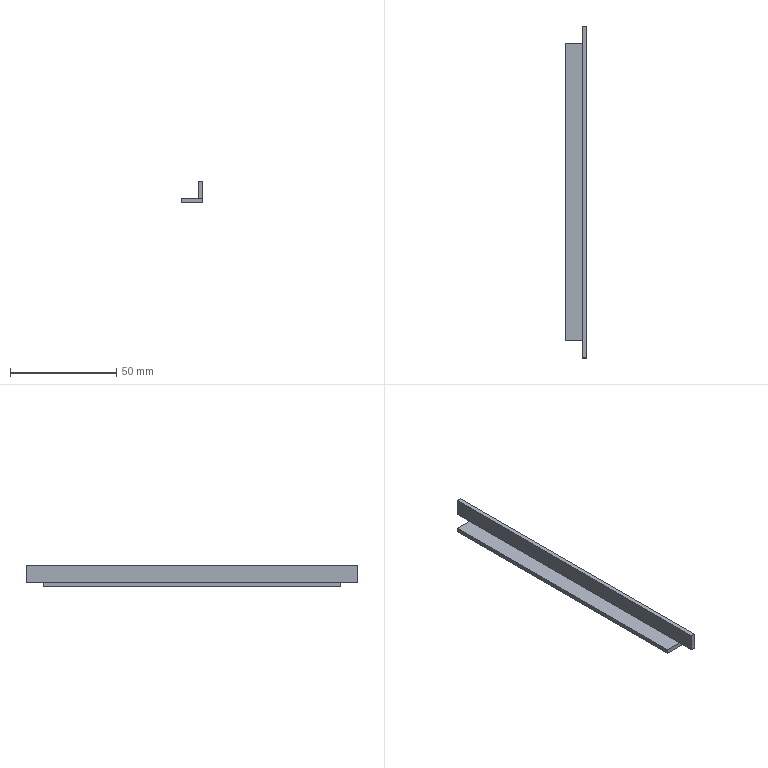Part | STEP file | 1-43.7 | 1 solid | 12 faces | box 10 x 156 x 10 mm | volume 5296 mm3 | plane 12
STEP:
#1=CARTESIAN_POINT('',(0.,0.,0.));
#2=DIRECTION('',(0.,0.,1.));
#3=DIRECTION('',(1.,0.,0.));
#4=AXIS2_PLACEMENT_3D('',#1,#2,#3);
#5=CARTESIAN_POINT('',(3.,-78.,-3.));
#6=VERTEX_POINT('',#5);
#7=CARTESIAN_POINT('',(3.,-78.,5.));
#8=VERTEX_POINT('',#7);
#9=CARTESIAN_POINT('',(3.,-78.,-3.));
#10=DIRECTION('',(0.,0.,1.));
#11=VECTOR('',#10,1.);
#12=LINE('',#9,#11);
#13=CARTESIAN_POINT('',(3.,0.,1.));
#14=DIRECTION('',(-1.,0.,0.));
#15=DIRECTION('',(0.,0.,1.));
#16=AXIS2_PLACEMENT_3D('',#13,#14,#15);
#17=PLANE('',#16);
#18=CARTESIAN_POINT('',(-4.,-78.));
#19=DIRECTION('',(1.,0.));
#20=VECTOR('',#19,1.);
#21=LINE('',#18,#20);
#22=(GEOMETRIC_REPRESENTATION_CONTEXT(2)PARAMETRIC_REPRESENTATION_CONTEXT()REPRESENTATION_CONTEXT('',''));
#23=DEFINITIONAL_REPRESENTATION('',(#21),#22);
#24=PCURVE('',#17,#23);
#25=CARTESIAN_POINT('',(0.,-78.,0.));
#26=DIRECTION('',(0.,1.,0.));
#27=DIRECTION('',(-1.,0.,0.));
#28=AXIS2_PLACEMENT_3D('',#25,#26,#27);
#29=PLANE('',#28);
#30=CARTESIAN_POINT('',(-3.,-3.));
#31=DIRECTION('',(0.,1.));
#32=VECTOR('',#31,1.);
#33=LINE('',#30,#32);
#34=(GEOMETRIC_REPRESENTATION_CONTEXT(2)PARAMETRIC_REPRESENTATION_CONTEXT()REPRESENTATION_CONTEXT('',''));
#35=DEFINITIONAL_REPRESENTATION('',(#33),#34);
#36=PCURVE('',#29,#35);
#37=SURFACE_CURVE('',#12,(#24,#36),.PCURVE_S1.);
#38=EDGE_CURVE('',#6,#8,#37,.T.);
#39=ORIENTED_EDGE('',*,*,#38,.T.);
#40=CARTESIAN_POINT('',(3.,78.,5.));
#41=VERTEX_POINT('',#40);
#42=CARTESIAN_POINT('',(3.,-78.,5.));
#43=DIRECTION('',(0.,1.,0.));
#44=VECTOR('',#43,1.);
#45=LINE('',#42,#44);
#46=CARTESIAN_POINT('',(4.,-78.));
#47=DIRECTION('',(0.,1.));
#48=VECTOR('',#47,1.);
#49=LINE('',#46,#48);
#50=(GEOMETRIC_REPRESENTATION_CONTEXT(2)PARAMETRIC_REPRESENTATION_CONTEXT()REPRESENTATION_CONTEXT('',''));
#51=DEFINITIONAL_REPRESENTATION('',(#49),#50);
#52=PCURVE('',#17,#51);
#53=CARTESIAN_POINT('',(4.,0.,5.));
#54=DIRECTION('',(0.,0.,1.));
#55=DIRECTION('',(1.,0.,0.));
#56=AXIS2_PLACEMENT_3D('',#53,#54,#55);
#57=PLANE('',#56);
#58=CARTESIAN_POINT('',(-1.,-78.));
#59=DIRECTION('',(0.,1.));
#60=VECTOR('',#59,1.);
#61=LINE('',#58,#60);
#62=(GEOMETRIC_REPRESENTATION_CONTEXT(2)PARAMETRIC_REPRESENTATION_CONTEXT()REPRESENTATION_CONTEXT('',''));
#63=DEFINITIONAL_REPRESENTATION('',(#61),#62);
#64=PCURVE('',#57,#63);
#65=SURFACE_CURVE('',#45,(#52,#64),.PCURVE_S1.);
#66=EDGE_CURVE('',#8,#41,#65,.T.);
#67=ORIENTED_EDGE('',*,*,#66,.T.);
#68=CARTESIAN_POINT('',(3.,78.,-3.));
#69=VERTEX_POINT('',#68);
#70=CARTESIAN_POINT('',(3.,78.,-3.));
#71=DIRECTION('',(0.,0.,1.));
#72=VECTOR('',#71,1.);
#73=LINE('',#70,#72);
#74=CARTESIAN_POINT('',(-4.,78.));
#75=DIRECTION('',(1.,0.));
#76=VECTOR('',#75,1.);
#77=LINE('',#74,#76);
#78=(GEOMETRIC_REPRESENTATION_CONTEXT(2)PARAMETRIC_REPRESENTATION_CONTEXT()REPRESENTATION_CONTEXT('',''));
#79=DEFINITIONAL_REPRESENTATION('',(#77),#78);
#80=PCURVE('',#17,#79);
#81=CARTESIAN_POINT('',(0.,78.,0.));
#82=DIRECTION('',(0.,1.,0.));
#83=DIRECTION('',(-1.,0.,0.));
#84=AXIS2_PLACEMENT_3D('',#81,#82,#83);
#85=PLANE('',#84);
#86=CARTESIAN_POINT('',(-3.,-3.));
#87=DIRECTION('',(0.,1.));
#88=VECTOR('',#87,1.);
#89=LINE('',#86,#88);
#90=(GEOMETRIC_REPRESENTATION_CONTEXT(2)PARAMETRIC_REPRESENTATION_CONTEXT()REPRESENTATION_CONTEXT('',''));
#91=DEFINITIONAL_REPRESENTATION('',(#89),#90);
#92=PCURVE('',#85,#91);
#93=SURFACE_CURVE('',#73,(#80,#92),.PCURVE_S1.);
#94=EDGE_CURVE('',#69,#41,#93,.T.);
#95=ORIENTED_EDGE('',*,*,#94,.F.);
#96=CARTESIAN_POINT('',(3.,70.,-3.));
#97=VERTEX_POINT('',#96);
#98=CARTESIAN_POINT('',(3.,70.,-3.));
#99=DIRECTION('',(0.,1.,0.));
#100=VECTOR('',#99,1.);
#101=LINE('',#98,#100);
#102=CARTESIAN_POINT('',(-4.,70.));
#103=DIRECTION('',(0.,1.));
#104=VECTOR('',#103,1.);
#105=LINE('',#102,#104);
#106=(GEOMETRIC_REPRESENTATION_CONTEXT(2)PARAMETRIC_REPRESENTATION_CONTEXT()REPRESENTATION_CONTEXT('',''));
#107=DEFINITIONAL_REPRESENTATION('',(#105),#106);
#108=PCURVE('',#17,#107);
#109=CARTESIAN_POINT('',(0.,74.,-3.));
#110=DIRECTION('',(0.,0.,1.));
#111=DIRECTION('',(0.,1.,0.));
#112=AXIS2_PLACEMENT_3D('',#109,#110,#111);
#113=PLANE('',#112);
#114=CARTESIAN_POINT('',(-4.,-3.));
#115=DIRECTION('',(1.,0.));
#116=VECTOR('',#115,1.);
#117=LINE('',#114,#116);
#118=(GEOMETRIC_REPRESENTATION_CONTEXT(2)PARAMETRIC_REPRESENTATION_CONTEXT()REPRESENTATION_CONTEXT('',''));
#119=DEFINITIONAL_REPRESENTATION('',(#117),#118);
#120=PCURVE('',#113,#119);
#121=SURFACE_CURVE('',#101,(#108,#120),.PCURVE_S1.);
#122=EDGE_CURVE('',#97,#69,#121,.T.);
#123=ORIENTED_EDGE('',*,*,#122,.F.);
#124=CARTESIAN_POINT('',(3.,-70.,-3.));
#125=VERTEX_POINT('',#124);
#126=CARTESIAN_POINT('',(3.,-70.,-3.));
#127=DIRECTION('',(0.,1.,0.));
#128=VECTOR('',#127,1.);
#129=LINE('',#126,#128);
#130=CARTESIAN_POINT('',(-4.,-70.));
#131=DIRECTION('',(0.,1.));
#132=VECTOR('',#131,1.);
#133=LINE('',#130,#132);
#134=(GEOMETRIC_REPRESENTATION_CONTEXT(2)PARAMETRIC_REPRESENTATION_CONTEXT()REPRESENTATION_CONTEXT('',''));
#135=DEFINITIONAL_REPRESENTATION('',(#133),#134);
#136=PCURVE('',#17,#135);
#137=CARTESIAN_POINT('',(-1.,0.,-3.));
#138=DIRECTION('',(0.,0.,1.));
#139=DIRECTION('',(1.,0.,0.));
#140=AXIS2_PLACEMENT_3D('',#137,#138,#139);
#141=PLANE('',#140);
#142=CARTESIAN_POINT('',(4.,-70.));
#143=DIRECTION('',(0.,1.));
#144=VECTOR('',#143,1.);
#145=LINE('',#142,#144);
#146=(GEOMETRIC_REPRESENTATION_CONTEXT(2)PARAMETRIC_REPRESENTATION_CONTEXT()REPRESENTATION_CONTEXT('',''));
#147=DEFINITIONAL_REPRESENTATION('',(#145),#146);
#148=PCURVE('',#141,#147);
#149=SURFACE_CURVE('',#129,(#136,#148),.PCURVE_S1.);
#150=EDGE_CURVE('',#125,#97,#149,.T.);
#151=ORIENTED_EDGE('',*,*,#150,.F.);
#152=CARTESIAN_POINT('',(3.,-78.,-3.));
#153=DIRECTION('',(0.,1.,0.));
#154=VECTOR('',#153,1.);
#155=LINE('',#152,#154);
#156=CARTESIAN_POINT('',(-4.,-78.));
#157=DIRECTION('',(0.,1.));
#158=VECTOR('',#157,1.);
#159=LINE('',#156,#158);
#160=(GEOMETRIC_REPRESENTATION_CONTEXT(2)PARAMETRIC_REPRESENTATION_CONTEXT()REPRESENTATION_CONTEXT('',''));
#161=DEFINITIONAL_REPRESENTATION('',(#159),#160);
#162=PCURVE('',#17,#161);
#163=CARTESIAN_POINT('',(0.,-74.,-3.));
#164=DIRECTION('',(0.,0.,1.));
#165=DIRECTION('',(0.,1.,0.));
#166=AXIS2_PLACEMENT_3D('',#163,#164,#165);
#167=PLANE('',#166);
#168=CARTESIAN_POINT('',(-4.,-3.));
#169=DIRECTION('',(1.,0.));
#170=VECTOR('',#169,1.);
#171=LINE('',#168,#170);
#172=(GEOMETRIC_REPRESENTATION_CONTEXT(2)PARAMETRIC_REPRESENTATION_CONTEXT()REPRESENTATION_CONTEXT('',''));
#173=DEFINITIONAL_REPRESENTATION('',(#171),#172);
#174=PCURVE('',#167,#173);
#175=SURFACE_CURVE('',#155,(#162,#174),.PCURVE_S1.);
#176=EDGE_CURVE('',#6,#125,#175,.T.);
#177=ORIENTED_EDGE('',*,*,#176,.F.);
#178=EDGE_LOOP('',(#39,#67,#95,#123,#151,#177));
#179=FACE_BOUND('',#178,.T.);
#180=ADVANCED_FACE('',(#179),#17,.T.);
#181=CARTESIAN_POINT('',(5.,-78.,5.));
#182=VERTEX_POINT('',#181);
#183=CARTESIAN_POINT('',(3.,-78.,5.));
#184=DIRECTION('',(1.,0.,0.));
#185=VECTOR('',#184,1.);
#186=LINE('',#183,#185);
#187=CARTESIAN_POINT('',(-1.,-78.));
#188=DIRECTION('',(1.,0.));
#189=VECTOR('',#188,1.);
#190=LINE('',#187,#189);
#191=(GEOMETRIC_REPRESENTATION_CONTEXT(2)PARAMETRIC_REPRESENTATION_CONTEXT()REPRESENTATION_CONTEXT('',''));
#192=DEFINITIONAL_REPRESENTATION('',(#190),#191);
#193=PCURVE('',#57,#192);
#194=CARTESIAN_POINT('',(-3.,5.));
#195=DIRECTION('',(-1.,0.));
#196=VECTOR('',#195,1.);
#197=LINE('',#194,#196);
#198=(GEOMETRIC_REPRESENTATION_CONTEXT(2)PARAMETRIC_REPRESENTATION_CONTEXT()REPRESENTATION_CONTEXT('',''));
#199=DEFINITIONAL_REPRESENTATION('',(#197),#198);
#200=PCURVE('',#29,#199);
#201=SURFACE_CURVE('',#186,(#193,#200),.PCURVE_S1.);
#202=EDGE_CURVE('',#8,#182,#201,.T.);
#203=ORIENTED_EDGE('',*,*,#202,.T.);
#204=CARTESIAN_POINT('',(5.,78.,5.));
#205=VERTEX_POINT('',#204);
#206=CARTESIAN_POINT('',(5.,-78.,5.));
#207=DIRECTION('',(0.,1.,0.));
#208=VECTOR('',#207,1.);
#209=LINE('',#206,#208);
#210=CARTESIAN_POINT('',(1.,-78.));
#211=DIRECTION('',(0.,1.));
#212=VECTOR('',#211,1.);
#213=LINE('',#210,#212);
#214=(GEOMETRIC_REPRESENTATION_CONTEXT(2)PARAMETRIC_REPRESENTATION_CONTEXT()REPRESENTATION_CONTEXT('',''));
#215=DEFINITIONAL_REPRESENTATION('',(#213),#214);
#216=PCURVE('',#57,#215);
#217=CARTESIAN_POINT('',(5.,0.,0.));
#218=DIRECTION('',(1.,0.,0.));
#219=DIRECTION('',(0.,0.,-1.));
#220=AXIS2_PLACEMENT_3D('',#217,#218,#219);
#221=PLANE('',#220);
#222=CARTESIAN_POINT('',(-5.,-78.));
#223=DIRECTION('',(0.,1.));
#224=VECTOR('',#223,1.);
#225=LINE('',#222,#224);
#226=(GEOMETRIC_REPRESENTATION_CONTEXT(2)PARAMETRIC_REPRESENTATION_CONTEXT()REPRESENTATION_CONTEXT('',''));
#227=DEFINITIONAL_REPRESENTATION('',(#225),#226);
#228=PCURVE('',#221,#227);
#229=SURFACE_CURVE('',#209,(#216,#228),.PCURVE_S1.);
#230=EDGE_CURVE('',#182,#205,#229,.T.);
#231=ORIENTED_EDGE('',*,*,#230,.T.);
#232=CARTESIAN_POINT('',(3.,78.,5.));
#233=DIRECTION('',(1.,0.,0.));
#234=VECTOR('',#233,1.);
#235=LINE('',#232,#234);
#236=CARTESIAN_POINT('',(-1.,78.));
#237=DIRECTION('',(1.,0.));
#238=VECTOR('',#237,1.);
#239=LINE('',#236,#238);
#240=(GEOMETRIC_REPRESENTATION_CONTEXT(2)PARAMETRIC_REPRESENTATION_CONTEXT()REPRESENTATION_CONTEXT('',''));
#241=DEFINITIONAL_REPRESENTATION('',(#239),#240);
#242=PCURVE('',#57,#241);
#243=CARTESIAN_POINT('',(-3.,5.));
#244=DIRECTION('',(-1.,0.));
#245=VECTOR('',#244,1.);
#246=LINE('',#243,#245);
#247=(GEOMETRIC_REPRESENTATION_CONTEXT(2)PARAMETRIC_REPRESENTATION_CONTEXT()REPRESENTATION_CONTEXT('',''));
#248=DEFINITIONAL_REPRESENTATION('',(#246),#247);
#249=PCURVE('',#85,#248);
#250=SURFACE_CURVE('',#235,(#242,#249),.PCURVE_S1.);
#251=EDGE_CURVE('',#41,#205,#250,.T.);
#252=ORIENTED_EDGE('',*,*,#251,.F.);
#253=ORIENTED_EDGE('',*,*,#66,.F.);
#254=EDGE_LOOP('',(#203,#231,#252,#253));
#255=FACE_BOUND('',#254,.T.);
#256=ADVANCED_FACE('',(#255),#57,.T.);
#257=ORIENTED_EDGE('',*,*,#38,.T.);
#258=ORIENTED_EDGE('',*,*,#202,.T.);
#259=CARTESIAN_POINT('',(5.,-78.,-3.));
#260=VERTEX_POINT('',#259);
#261=CARTESIAN_POINT('',(5.,-78.,5.));
#262=DIRECTION('',(0.,0.,-1.));
#263=VECTOR('',#262,1.);
#264=LINE('',#261,#263);
#265=CARTESIAN_POINT('',(-5.,5.));
#266=DIRECTION('',(0.,-1.));
#267=VECTOR('',#266,1.);
#268=LINE('',#265,#267);
#269=(GEOMETRIC_REPRESENTATION_CONTEXT(2)PARAMETRIC_REPRESENTATION_CONTEXT()REPRESENTATION_CONTEXT('',''));
#270=DEFINITIONAL_REPRESENTATION('',(#268),#269);
#271=PCURVE('',#29,#270);
#272=CARTESIAN_POINT('',(-5.,-78.));
#273=DIRECTION('',(1.,0.));
#274=VECTOR('',#273,1.);
#275=LINE('',#272,#274);
#276=(GEOMETRIC_REPRESENTATION_CONTEXT(2)PARAMETRIC_REPRESENTATION_CONTEXT()REPRESENTATION_CONTEXT('',''));
#277=DEFINITIONAL_REPRESENTATION('',(#275),#276);
#278=PCURVE('',#221,#277);
#279=SURFACE_CURVE('',#264,(#271,#278),.PCURVE_S1.);
#280=EDGE_CURVE('',#182,#260,#279,.T.);
#281=ORIENTED_EDGE('',*,*,#280,.T.);
#282=CARTESIAN_POINT('',(5.,-78.,-3.));
#283=DIRECTION('',(-1.,0.,0.));
#284=VECTOR('',#283,1.);
#285=LINE('',#282,#284);
#286=CARTESIAN_POINT('',(-5.,-3.));
#287=DIRECTION('',(1.,0.));
#288=VECTOR('',#287,1.);
#289=LINE('',#286,#288);
#290=(GEOMETRIC_REPRESENTATION_CONTEXT(2)PARAMETRIC_REPRESENTATION_CONTEXT()REPRESENTATION_CONTEXT('',''));
#291=DEFINITIONAL_REPRESENTATION('',(#289),#290);
#292=PCURVE('',#29,#291);
#293=CARTESIAN_POINT('',(-4.,-5.));
#294=DIRECTION('',(0.,1.));
#295=VECTOR('',#294,1.);
#296=LINE('',#293,#295);
#297=(GEOMETRIC_REPRESENTATION_CONTEXT(2)PARAMETRIC_REPRESENTATION_CONTEXT()REPRESENTATION_CONTEXT('',''));
#298=DEFINITIONAL_REPRESENTATION('',(#296),#297);
#299=PCURVE('',#167,#298);
#300=SURFACE_CURVE('',#285,(#292,#299),.PCURVE_S1.);
#301=EDGE_CURVE('',#260,#6,#300,.T.);
#302=ORIENTED_EDGE('',*,*,#301,.T.);
#303=EDGE_LOOP('',(#257,#258,#281,#302));
#304=FACE_BOUND('',#303,.F.);
#305=ADVANCED_FACE('',(#304),#29,.F.);
#306=ORIENTED_EDGE('',*,*,#94,.T.);
#307=ORIENTED_EDGE('',*,*,#251,.T.);
#308=CARTESIAN_POINT('',(5.,78.,-3.));
#309=VERTEX_POINT('',#308);
#310=CARTESIAN_POINT('',(5.,78.,5.));
#311=DIRECTION('',(0.,0.,-1.));
#312=VECTOR('',#311,1.);
#313=LINE('',#310,#312);
#314=CARTESIAN_POINT('',(-5.,5.));
#315=DIRECTION('',(0.,-1.));
#316=VECTOR('',#315,1.);
#317=LINE('',#314,#316);
#318=(GEOMETRIC_REPRESENTATION_CONTEXT(2)PARAMETRIC_REPRESENTATION_CONTEXT()REPRESENTATION_CONTEXT('',''));
#319=DEFINITIONAL_REPRESENTATION('',(#317),#318);
#320=PCURVE('',#85,#319);
#321=CARTESIAN_POINT('',(-5.,78.));
#322=DIRECTION('',(1.,0.));
#323=VECTOR('',#322,1.);
#324=LINE('',#321,#323);
#325=(GEOMETRIC_REPRESENTATION_CONTEXT(2)PARAMETRIC_REPRESENTATION_CONTEXT()REPRESENTATION_CONTEXT('',''));
#326=DEFINITIONAL_REPRESENTATION('',(#324),#325);
#327=PCURVE('',#221,#326);
#328=SURFACE_CURVE('',#313,(#320,#327),.PCURVE_S1.);
#329=EDGE_CURVE('',#205,#309,#328,.T.);
#330=ORIENTED_EDGE('',*,*,#329,.T.);
#331=CARTESIAN_POINT('',(5.,78.,-3.));
#332=DIRECTION('',(-1.,0.,0.));
#333=VECTOR('',#332,1.);
#334=LINE('',#331,#333);
#335=CARTESIAN_POINT('',(-5.,-3.));
#336=DIRECTION('',(1.,0.));
#337=VECTOR('',#336,1.);
#338=LINE('',#335,#337);
#339=(GEOMETRIC_REPRESENTATION_CONTEXT(2)PARAMETRIC_REPRESENTATION_CONTEXT()REPRESENTATION_CONTEXT('',''));
#340=DEFINITIONAL_REPRESENTATION('',(#338),#339);
#341=PCURVE('',#85,#340);
#342=CARTESIAN_POINT('',(4.,-5.));
#343=DIRECTION('',(0.,1.));
#344=VECTOR('',#343,1.);
#345=LINE('',#342,#344);
#346=(GEOMETRIC_REPRESENTATION_CONTEXT(2)PARAMETRIC_REPRESENTATION_CONTEXT()REPRESENTATION_CONTEXT('',''));
#347=DEFINITIONAL_REPRESENTATION('',(#345),#346);
#348=PCURVE('',#113,#347);
#349=SURFACE_CURVE('',#334,(#341,#348),.PCURVE_S1.);
#350=EDGE_CURVE('',#309,#69,#349,.T.);
#351=ORIENTED_EDGE('',*,*,#350,.T.);
#352=EDGE_LOOP('',(#306,#307,#330,#351));
#353=FACE_BOUND('',#352,.T.);
#354=ADVANCED_FACE('',(#353),#85,.T.);
#355=CARTESIAN_POINT('',(-5.,-70.,-5.));
#356=VERTEX_POINT('',#355);
#357=CARTESIAN_POINT('',(-5.,70.,-5.));
#358=VERTEX_POINT('',#357);
#359=CARTESIAN_POINT('',(-5.,-70.,-5.));
#360=DIRECTION('',(0.,1.,0.));
#361=VECTOR('',#360,1.);
#362=LINE('',#359,#361);
#363=CARTESIAN_POINT('',(0.,0.,-5.));
#364=DIRECTION('',(0.,0.,-1.));
#365=DIRECTION('',(-1.,0.,0.));
#366=AXIS2_PLACEMENT_3D('',#363,#364,#365);
#367=PLANE('',#366);
#368=CARTESIAN_POINT('',(5.,-70.));
#369=DIRECTION('',(0.,1.));
#370=VECTOR('',#369,1.);
#371=LINE('',#368,#370);
#372=(GEOMETRIC_REPRESENTATION_CONTEXT(2)PARAMETRIC_REPRESENTATION_CONTEXT()REPRESENTATION_CONTEXT('',''));
#373=DEFINITIONAL_REPRESENTATION('',(#371),#372);
#374=PCURVE('',#367,#373);
#375=CARTESIAN_POINT('',(-5.,0.,-4.));
#376=DIRECTION('',(-1.,0.,0.));
#377=DIRECTION('',(0.,0.,1.));
#378=AXIS2_PLACEMENT_3D('',#375,#376,#377);
#379=PLANE('',#378);
#380=CARTESIAN_POINT('',(-1.,-70.));
#381=DIRECTION('',(0.,1.));
#382=VECTOR('',#381,1.);
#383=LINE('',#380,#382);
#384=(GEOMETRIC_REPRESENTATION_CONTEXT(2)PARAMETRIC_REPRESENTATION_CONTEXT()REPRESENTATION_CONTEXT('',''));
#385=DEFINITIONAL_REPRESENTATION('',(#383),#384);
#386=PCURVE('',#379,#385);
#387=SURFACE_CURVE('',#362,(#374,#386),.PCURVE_S1.);
#388=EDGE_CURVE('',#356,#358,#387,.T.);
#389=ORIENTED_EDGE('',*,*,#388,.T.);
#390=CARTESIAN_POINT('',(5.,70.,-5.));
#391=VERTEX_POINT('',#390);
#392=CARTESIAN_POINT('',(5.,70.,-5.));
#393=DIRECTION('',(-1.,0.,0.));
#394=VECTOR('',#393,1.);
#395=LINE('',#392,#394);
#396=CARTESIAN_POINT('',(-5.,70.));
#397=DIRECTION('',(1.,0.));
#398=VECTOR('',#397,1.);
#399=LINE('',#396,#398);
#400=(GEOMETRIC_REPRESENTATION_CONTEXT(2)PARAMETRIC_REPRESENTATION_CONTEXT()REPRESENTATION_CONTEXT('',''));
#401=DEFINITIONAL_REPRESENTATION('',(#399),#400);
#402=PCURVE('',#367,#401);
#403=CARTESIAN_POINT('',(0.,70.,-4.));
#404=DIRECTION('',(0.,-1.,0.));
#405=DIRECTION('',(0.,0.,1.));
#406=AXIS2_PLACEMENT_3D('',#403,#404,#405);
#407=PLANE('',#406);
#408=CARTESIAN_POINT('',(-1.,-5.));
#409=DIRECTION('',(0.,1.));
#410=VECTOR('',#409,1.);
#411=LINE('',#408,#410);
#412=(GEOMETRIC_REPRESENTATION_CONTEXT(2)PARAMETRIC_REPRESENTATION_CONTEXT()REPRESENTATION_CONTEXT('',''));
#413=DEFINITIONAL_REPRESENTATION('',(#411),#412);
#414=PCURVE('',#407,#413);
#415=SURFACE_CURVE('',#395,(#402,#414),.PCURVE_S1.);
#416=EDGE_CURVE('',#391,#358,#415,.T.);
#417=ORIENTED_EDGE('',*,*,#416,.F.);
#418=CARTESIAN_POINT('',(5.,-70.,-5.));
#419=VERTEX_POINT('',#418);
#420=CARTESIAN_POINT('',(5.,-70.,-5.));
#421=DIRECTION('',(0.,1.,0.));
#422=VECTOR('',#421,1.);
#423=LINE('',#420,#422);
#424=CARTESIAN_POINT('',(-5.,-70.));
#425=DIRECTION('',(0.,1.));
#426=VECTOR('',#425,1.);
#427=LINE('',#424,#426);
#428=(GEOMETRIC_REPRESENTATION_CONTEXT(2)PARAMETRIC_REPRESENTATION_CONTEXT()REPRESENTATION_CONTEXT('',''));
#429=DEFINITIONAL_REPRESENTATION('',(#427),#428);
#430=PCURVE('',#367,#429);
#431=CARTESIAN_POINT('',(5.,-70.));
#432=DIRECTION('',(0.,1.));
#433=VECTOR('',#432,1.);
#434=LINE('',#431,#433);
#435=(GEOMETRIC_REPRESENTATION_CONTEXT(2)PARAMETRIC_REPRESENTATION_CONTEXT()REPRESENTATION_CONTEXT('',''));
#436=DEFINITIONAL_REPRESENTATION('',(#434),#435);
#437=PCURVE('',#221,#436);
#438=SURFACE_CURVE('',#423,(#430,#437),.PCURVE_S1.);
#439=EDGE_CURVE('',#419,#391,#438,.T.);
#440=ORIENTED_EDGE('',*,*,#439,.F.);
#441=CARTESIAN_POINT('',(5.,-70.,-5.));
#442=DIRECTION('',(-1.,0.,0.));
#443=VECTOR('',#442,1.);
#444=LINE('',#441,#443);
#445=CARTESIAN_POINT('',(-5.,-70.));
#446=DIRECTION('',(1.,0.));
#447=VECTOR('',#446,1.);
#448=LINE('',#445,#447);
#449=(GEOMETRIC_REPRESENTATION_CONTEXT(2)PARAMETRIC_REPRESENTATION_CONTEXT()REPRESENTATION_CONTEXT('',''));
#450=DEFINITIONAL_REPRESENTATION('',(#448),#449);
#451=PCURVE('',#367,#450);
#452=CARTESIAN_POINT('',(0.,-70.,-4.));
#453=DIRECTION('',(0.,1.,0.));
#454=DIRECTION('',(0.,0.,-1.));
#455=AXIS2_PLACEMENT_3D('',#452,#453,#454);
#456=PLANE('',#455);
#457=CARTESIAN_POINT('',(1.,-5.));
#458=DIRECTION('',(0.,1.));
#459=VECTOR('',#458,1.);
#460=LINE('',#457,#459);
#461=(GEOMETRIC_REPRESENTATION_CONTEXT(2)PARAMETRIC_REPRESENTATION_CONTEXT()REPRESENTATION_CONTEXT('',''));
#462=DEFINITIONAL_REPRESENTATION('',(#460),#461);
#463=PCURVE('',#456,#462);
#464=SURFACE_CURVE('',#444,(#451,#463),.PCURVE_S1.);
#465=EDGE_CURVE('',#419,#356,#464,.T.);
#466=ORIENTED_EDGE('',*,*,#465,.T.);
#467=EDGE_LOOP('',(#389,#417,#440,#466));
#468=FACE_BOUND('',#467,.T.);
#469=ADVANCED_FACE('',(#468),#367,.T.);
#470=CARTESIAN_POINT('',(-5.,-70.,-3.));
#471=VERTEX_POINT('',#470);
#472=CARTESIAN_POINT('',(-5.,70.,-3.));
#473=VERTEX_POINT('',#472);
#474=CARTESIAN_POINT('',(-5.,-70.,-3.));
#475=DIRECTION('',(0.,1.,0.));
#476=VECTOR('',#475,1.);
#477=LINE('',#474,#476);
#478=CARTESIAN_POINT('',(1.,-70.));
#479=DIRECTION('',(0.,1.));
#480=VECTOR('',#479,1.);
#481=LINE('',#478,#480);
#482=(GEOMETRIC_REPRESENTATION_CONTEXT(2)PARAMETRIC_REPRESENTATION_CONTEXT()REPRESENTATION_CONTEXT('',''));
#483=DEFINITIONAL_REPRESENTATION('',(#481),#482);
#484=PCURVE('',#379,#483);
#485=CARTESIAN_POINT('',(-4.,-70.));
#486=DIRECTION('',(0.,1.));
#487=VECTOR('',#486,1.);
#488=LINE('',#485,#487);
#489=(GEOMETRIC_REPRESENTATION_CONTEXT(2)PARAMETRIC_REPRESENTATION_CONTEXT()REPRESENTATION_CONTEXT('',''));
#490=DEFINITIONAL_REPRESENTATION('',(#488),#489);
#491=PCURVE('',#141,#490);
#492=SURFACE_CURVE('',#477,(#484,#491),.PCURVE_S1.);
#493=EDGE_CURVE('',#471,#473,#492,.T.);
#494=ORIENTED_EDGE('',*,*,#493,.T.);
#495=CARTESIAN_POINT('',(-5.,70.,-5.));
#496=DIRECTION('',(0.,0.,1.));
#497=VECTOR('',#496,1.);
#498=LINE('',#495,#497);
#499=CARTESIAN_POINT('',(-1.,70.));
#500=DIRECTION('',(1.,0.));
#501=VECTOR('',#500,1.);
#502=LINE('',#499,#501);
#503=(GEOMETRIC_REPRESENTATION_CONTEXT(2)PARAMETRIC_REPRESENTATION_CONTEXT()REPRESENTATION_CONTEXT('',''));
#504=DEFINITIONAL_REPRESENTATION('',(#502),#503);
#505=PCURVE('',#379,#504);
#506=CARTESIAN_POINT('',(-1.,5.));
#507=DIRECTION('',(1.,0.));
#508=VECTOR('',#507,1.);
#509=LINE('',#506,#508);
#510=(GEOMETRIC_REPRESENTATION_CONTEXT(2)PARAMETRIC_REPRESENTATION_CONTEXT()REPRESENTATION_CONTEXT('',''));
#511=DEFINITIONAL_REPRESENTATION('',(#509),#510);
#512=PCURVE('',#407,#511);
#513=SURFACE_CURVE('',#498,(#505,#512),.PCURVE_S1.);
#514=EDGE_CURVE('',#358,#473,#513,.T.);
#515=ORIENTED_EDGE('',*,*,#514,.F.);
#516=ORIENTED_EDGE('',*,*,#388,.F.);
#517=CARTESIAN_POINT('',(-5.,-70.,-3.));
#518=DIRECTION('',(0.,0.,-1.));
#519=VECTOR('',#518,1.);
#520=LINE('',#517,#519);
#521=CARTESIAN_POINT('',(1.,-70.));
#522=DIRECTION('',(-1.,0.));
#523=VECTOR('',#522,1.);
#524=LINE('',#521,#523);
#525=(GEOMETRIC_REPRESENTATION_CONTEXT(2)PARAMETRIC_REPRESENTATION_CONTEXT()REPRESENTATION_CONTEXT('',''));
#526=DEFINITIONAL_REPRESENTATION('',(#524),#525);
#527=PCURVE('',#379,#526);
#528=CARTESIAN_POINT('',(-1.,5.));
#529=DIRECTION('',(1.,0.));
#530=VECTOR('',#529,1.);
#531=LINE('',#528,#530);
#532=(GEOMETRIC_REPRESENTATION_CONTEXT(2)PARAMETRIC_REPRESENTATION_CONTEXT()REPRESENTATION_CONTEXT('',''));
#533=DEFINITIONAL_REPRESENTATION('',(#531),#532);
#534=PCURVE('',#456,#533);
#535=SURFACE_CURVE('',#520,(#527,#534),.PCURVE_S1.);
#536=EDGE_CURVE('',#471,#356,#535,.T.);
#537=ORIENTED_EDGE('',*,*,#536,.F.);
#538=EDGE_LOOP('',(#494,#515,#516,#537));
#539=FACE_BOUND('',#538,.T.);
#540=ADVANCED_FACE('',(#539),#379,.T.);
#541=ORIENTED_EDGE('',*,*,#150,.T.);
#542=CARTESIAN_POINT('',(3.,70.,-3.));
#543=DIRECTION('',(-1.,0.,0.));
#544=VECTOR('',#543,1.);
#545=LINE('',#542,#544);
#546=CARTESIAN_POINT('',(4.,70.));
#547=DIRECTION('',(-1.,0.));
#548=VECTOR('',#547,1.);
#549=LINE('',#546,#548);
#550=(GEOMETRIC_REPRESENTATION_CONTEXT(2)PARAMETRIC_REPRESENTATION_CONTEXT()REPRESENTATION_CONTEXT('',''));
#551=DEFINITIONAL_REPRESENTATION('',(#549),#550);
#552=PCURVE('',#141,#551);
#553=CARTESIAN_POINT('',(1.,-3.));
#554=DIRECTION('',(0.,1.));
#555=VECTOR('',#554,1.);
#556=LINE('',#553,#555);
#557=(GEOMETRIC_REPRESENTATION_CONTEXT(2)PARAMETRIC_REPRESENTATION_CONTEXT()REPRESENTATION_CONTEXT('',''));
#558=DEFINITIONAL_REPRESENTATION('',(#556),#557);
#559=PCURVE('',#407,#558);
#560=SURFACE_CURVE('',#545,(#552,#559),.PCURVE_S1.);
#561=EDGE_CURVE('',#97,#473,#560,.T.);
#562=ORIENTED_EDGE('',*,*,#561,.T.);
#563=ORIENTED_EDGE('',*,*,#493,.F.);
#564=CARTESIAN_POINT('',(3.,-70.,-3.));
#565=DIRECTION('',(-1.,0.,0.));
#566=VECTOR('',#565,1.);
#567=LINE('',#564,#566);
#568=CARTESIAN_POINT('',(4.,-70.));
#569=DIRECTION('',(-1.,0.));
#570=VECTOR('',#569,1.);
#571=LINE('',#568,#570);
#572=(GEOMETRIC_REPRESENTATION_CONTEXT(2)PARAMETRIC_REPRESENTATION_CONTEXT()REPRESENTATION_CONTEXT('',''));
#573=DEFINITIONAL_REPRESENTATION('',(#571),#572);
#574=PCURVE('',#141,#573);
#575=CARTESIAN_POINT('',(-1.,-3.));
#576=DIRECTION('',(0.,1.));
#577=VECTOR('',#576,1.);
#578=LINE('',#575,#577);
#579=(GEOMETRIC_REPRESENTATION_CONTEXT(2)PARAMETRIC_REPRESENTATION_CONTEXT()REPRESENTATION_CONTEXT('',''));
#580=DEFINITIONAL_REPRESENTATION('',(#578),#579);
#581=PCURVE('',#456,#580);
#582=SURFACE_CURVE('',#567,(#574,#581),.PCURVE_S1.);
#583=EDGE_CURVE('',#125,#471,#582,.T.);
#584=ORIENTED_EDGE('',*,*,#583,.F.);
#585=EDGE_LOOP('',(#541,#562,#563,#584));
#586=FACE_BOUND('',#585,.T.);
#587=ADVANCED_FACE('',(#586),#141,.T.);
#588=ORIENTED_EDGE('',*,*,#280,.T.);
#589=CARTESIAN_POINT('',(5.,-70.,-3.));
#590=VERTEX_POINT('',#589);
#591=CARTESIAN_POINT('',(5.,-70.,-3.));
#592=DIRECTION('',(0.,-1.,0.));
#593=VECTOR('',#592,1.);
#594=LINE('',#591,#593);
#595=CARTESIAN_POINT('',(3.,-70.));
#596=DIRECTION('',(0.,-1.));
#597=VECTOR('',#596,1.);
#598=LINE('',#595,#597);
#599=(GEOMETRIC_REPRESENTATION_CONTEXT(2)PARAMETRIC_REPRESENTATION_CONTEXT()REPRESENTATION_CONTEXT('',''));
#600=DEFINITIONAL_REPRESENTATION('',(#598),#599);
#601=PCURVE('',#221,#600);
#602=CARTESIAN_POINT('',(4.,-5.));
#603=DIRECTION('',(-1.,0.));
#604=VECTOR('',#603,1.);
#605=LINE('',#602,#604);
#606=(GEOMETRIC_REPRESENTATION_CONTEXT(2)PARAMETRIC_REPRESENTATION_CONTEXT()REPRESENTATION_CONTEXT('',''));
#607=DEFINITIONAL_REPRESENTATION('',(#605),#606);
#608=PCURVE('',#167,#607);
#609=SURFACE_CURVE('',#594,(#601,#608),.PCURVE_S1.);
#610=EDGE_CURVE('',#590,#260,#609,.T.);
#611=ORIENTED_EDGE('',*,*,#610,.F.);
#612=CARTESIAN_POINT('',(5.,-70.,-5.));
#613=DIRECTION('',(0.,0.,1.));
#614=VECTOR('',#613,1.);
#615=LINE('',#612,#614);
#616=CARTESIAN_POINT('',(5.,-70.));
#617=DIRECTION('',(-1.,0.));
#618=VECTOR('',#617,1.);
#619=LINE('',#616,#618);
#620=(GEOMETRIC_REPRESENTATION_CONTEXT(2)PARAMETRIC_REPRESENTATION_CONTEXT()REPRESENTATION_CONTEXT('',''));
#621=DEFINITIONAL_REPRESENTATION('',(#619),#620);
#622=PCURVE('',#221,#621);
#623=CARTESIAN_POINT('',(1.,-5.));
#624=DIRECTION('',(-1.,0.));
#625=VECTOR('',#624,1.);
#626=LINE('',#623,#625);
#627=(GEOMETRIC_REPRESENTATION_CONTEXT(2)PARAMETRIC_REPRESENTATION_CONTEXT()REPRESENTATION_CONTEXT('',''));
#628=DEFINITIONAL_REPRESENTATION('',(#626),#627);
#629=PCURVE('',#456,#628);
#630=SURFACE_CURVE('',#615,(#622,#629),.PCURVE_S1.);
#631=EDGE_CURVE('',#419,#590,#630,.T.);
#632=ORIENTED_EDGE('',*,*,#631,.F.);
#633=ORIENTED_EDGE('',*,*,#439,.T.);
#634=CARTESIAN_POINT('',(5.,70.,-3.));
#635=VERTEX_POINT('',#634);
#636=CARTESIAN_POINT('',(5.,70.,-3.));
#637=DIRECTION('',(0.,0.,-1.));
#638=VECTOR('',#637,1.);
#639=LINE('',#636,#638);
#640=CARTESIAN_POINT('',(3.,70.));
#641=DIRECTION('',(1.,0.));
#642=VECTOR('',#641,1.);
#643=LINE('',#640,#642);
#644=(GEOMETRIC_REPRESENTATION_CONTEXT(2)PARAMETRIC_REPRESENTATION_CONTEXT()REPRESENTATION_CONTEXT('',''));
#645=DEFINITIONAL_REPRESENTATION('',(#643),#644);
#646=PCURVE('',#221,#645);
#647=CARTESIAN_POINT('',(1.,-5.));
#648=DIRECTION('',(-1.,0.));
#649=VECTOR('',#648,1.);
#650=LINE('',#647,#649);
#651=(GEOMETRIC_REPRESENTATION_CONTEXT(2)PARAMETRIC_REPRESENTATION_CONTEXT()REPRESENTATION_CONTEXT('',''));
#652=DEFINITIONAL_REPRESENTATION('',(#650),#651);
#653=PCURVE('',#407,#652);
#654=SURFACE_CURVE('',#639,(#646,#653),.PCURVE_S1.);
#655=EDGE_CURVE('',#635,#391,#654,.T.);
#656=ORIENTED_EDGE('',*,*,#655,.F.);
#657=CARTESIAN_POINT('',(5.,78.,-3.));
#658=DIRECTION('',(0.,-1.,0.));
#659=VECTOR('',#658,1.);
#660=LINE('',#657,#659);
#661=CARTESIAN_POINT('',(3.,78.));
#662=DIRECTION('',(0.,-1.));
#663=VECTOR('',#662,1.);
#664=LINE('',#661,#663);
#665=(GEOMETRIC_REPRESENTATION_CONTEXT(2)PARAMETRIC_REPRESENTATION_CONTEXT()REPRESENTATION_CONTEXT('',''));
#666=DEFINITIONAL_REPRESENTATION('',(#664),#665);
#667=PCURVE('',#221,#666);
#668=CARTESIAN_POINT('',(4.,-5.));
#669=DIRECTION('',(-1.,0.));
#670=VECTOR('',#669,1.);
#671=LINE('',#668,#670);
#672=(GEOMETRIC_REPRESENTATION_CONTEXT(2)PARAMETRIC_REPRESENTATION_CONTEXT()REPRESENTATION_CONTEXT('',''));
#673=DEFINITIONAL_REPRESENTATION('',(#671),#672);
#674=PCURVE('',#113,#673);
#675=SURFACE_CURVE('',#660,(#667,#674),.PCURVE_S1.);
#676=EDGE_CURVE('',#309,#635,#675,.T.);
#677=ORIENTED_EDGE('',*,*,#676,.F.);
#678=ORIENTED_EDGE('',*,*,#329,.F.);
#679=ORIENTED_EDGE('',*,*,#230,.F.);
#680=EDGE_LOOP('',(#588,#611,#632,#633,#656,#677,#678,#679));
#681=FACE_BOUND('',#680,.T.);
#682=ADVANCED_FACE('',(#681),#221,.T.);
#683=CARTESIAN_POINT('',(5.,70.,-3.));
#684=DIRECTION('',(-1.,0.,0.));
#685=VECTOR('',#684,1.);
#686=LINE('',#683,#685);
#687=CARTESIAN_POINT('',(-4.,-5.));
#688=DIRECTION('',(0.,1.));
#689=VECTOR('',#688,1.);
#690=LINE('',#687,#689);
#691=(GEOMETRIC_REPRESENTATION_CONTEXT(2)PARAMETRIC_REPRESENTATION_CONTEXT()REPRESENTATION_CONTEXT('',''));
#692=DEFINITIONAL_REPRESENTATION('',(#690),#691);
#693=PCURVE('',#113,#692);
#694=CARTESIAN_POINT('',(1.,-5.));
#695=DIRECTION('',(0.,1.));
#696=VECTOR('',#695,1.);
#697=LINE('',#694,#696);
#698=(GEOMETRIC_REPRESENTATION_CONTEXT(2)PARAMETRIC_REPRESENTATION_CONTEXT()REPRESENTATION_CONTEXT('',''));
#699=DEFINITIONAL_REPRESENTATION('',(#697),#698);
#700=PCURVE('',#407,#699);
#701=SURFACE_CURVE('',#686,(#693,#700),.PCURVE_S1.);
#702=EDGE_CURVE('',#635,#97,#701,.T.);
#703=ORIENTED_EDGE('',*,*,#702,.F.);
#704=ORIENTED_EDGE('',*,*,#676,.F.);
#705=ORIENTED_EDGE('',*,*,#350,.T.);
#706=ORIENTED_EDGE('',*,*,#122,.F.);
#707=EDGE_LOOP('',(#703,#704,#705,#706));
#708=FACE_BOUND('',#707,.F.);
#709=ADVANCED_FACE('',(#708),#113,.F.);
#710=ORIENTED_EDGE('',*,*,#301,.F.);
#711=ORIENTED_EDGE('',*,*,#610,.F.);
#712=CARTESIAN_POINT('',(5.,-70.,-3.));
#713=DIRECTION('',(-1.,0.,0.));
#714=VECTOR('',#713,1.);
#715=LINE('',#712,#714);
#716=CARTESIAN_POINT('',(4.,-5.));
#717=DIRECTION('',(0.,1.));
#718=VECTOR('',#717,1.);
#719=LINE('',#716,#718);
#720=(GEOMETRIC_REPRESENTATION_CONTEXT(2)PARAMETRIC_REPRESENTATION_CONTEXT()REPRESENTATION_CONTEXT('',''));
#721=DEFINITIONAL_REPRESENTATION('',(#719),#720);
#722=PCURVE('',#167,#721);
#723=CARTESIAN_POINT('',(-1.,-5.));
#724=DIRECTION('',(0.,1.));
#725=VECTOR('',#724,1.);
#726=LINE('',#723,#725);
#727=(GEOMETRIC_REPRESENTATION_CONTEXT(2)PARAMETRIC_REPRESENTATION_CONTEXT()REPRESENTATION_CONTEXT('',''));
#728=DEFINITIONAL_REPRESENTATION('',(#726),#727);
#729=PCURVE('',#456,#728);
#730=SURFACE_CURVE('',#715,(#722,#729),.PCURVE_S1.);
#731=EDGE_CURVE('',#590,#125,#730,.T.);
#732=ORIENTED_EDGE('',*,*,#731,.T.);
#733=ORIENTED_EDGE('',*,*,#176,.F.);
#734=EDGE_LOOP('',(#710,#711,#732,#733));
#735=FACE_BOUND('',#734,.F.);
#736=ADVANCED_FACE('',(#735),#167,.F.);
#737=ORIENTED_EDGE('',*,*,#416,.F.);
#738=ORIENTED_EDGE('',*,*,#655,.F.);
#739=ORIENTED_EDGE('',*,*,#702,.T.);
#740=ORIENTED_EDGE('',*,*,#561,.T.);
#741=ORIENTED_EDGE('',*,*,#514,.F.);
#742=EDGE_LOOP('',(#737,#738,#739,#740,#741));
#743=FACE_BOUND('',#742,.F.);
#744=ADVANCED_FACE('',(#743),#407,.F.);
#745=ORIENTED_EDGE('',*,*,#583,.F.);
#746=ORIENTED_EDGE('',*,*,#731,.F.);
#747=ORIENTED_EDGE('',*,*,#631,.F.);
#748=ORIENTED_EDGE('',*,*,#465,.T.);
#749=ORIENTED_EDGE('',*,*,#536,.F.);
#750=EDGE_LOOP('',(#745,#746,#747,#748,#749));
#751=FACE_BOUND('',#750,.F.);
#752=ADVANCED_FACE('',(#751),#456,.F.);
#753=CLOSED_SHELL('',(#180,#256,#305,#354,#469,#540,#587,#682,#709,#736,#744,#752));
#754=MANIFOLD_SOLID_BREP('',#753);
#755=(LENGTH_UNIT()NAMED_UNIT(*)SI_UNIT(.MILLI.,.METRE.));
#756=UNCERTAINTY_MEASURE_WITH_UNIT(LENGTH_MEASURE(0.0000001),#755,'','');
#757=(NAMED_UNIT(*)PLANE_ANGLE_UNIT()SI_UNIT($,.RADIAN.));
#758=(NAMED_UNIT(*)SI_UNIT($,.STERADIAN.)SOLID_ANGLE_UNIT());
#759=(GEOMETRIC_REPRESENTATION_CONTEXT(3)GLOBAL_UNCERTAINTY_ASSIGNED_CONTEXT((#756))GLOBAL_UNIT_ASSIGNED_CONTEXT((#755,#757,#758))REPRESENTATION_CONTEXT('',''));
#760=ADVANCED_BREP_SHAPE_REPRESENTATION('',(#4,#754),#759);